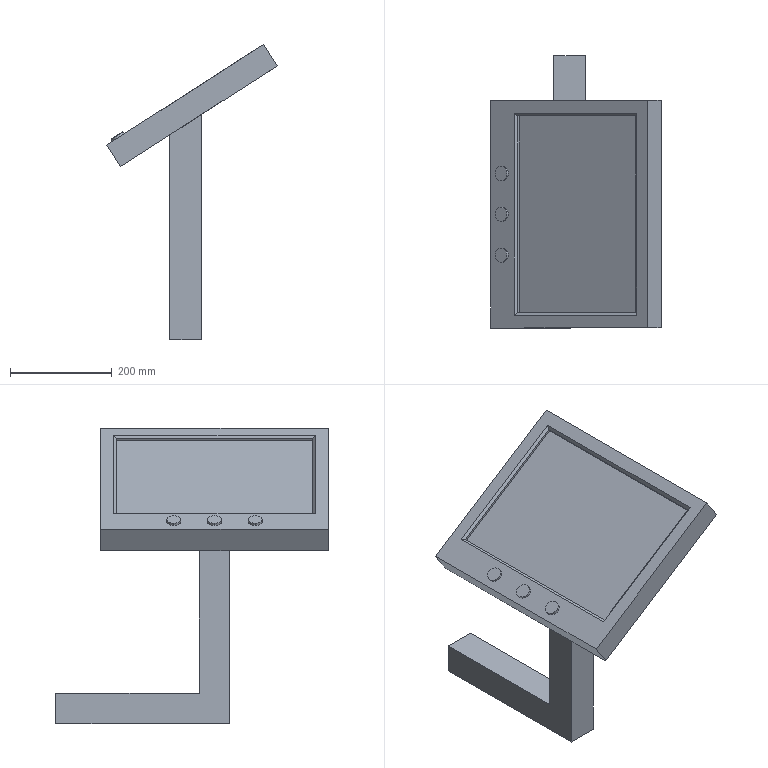Part | SolidWorks | features ICE 2, BossThin 1, Chamfer 1, Extrusion 1, MoveFace 1, Split 1 | 4 solids | 34 faces | box 334.254 x 534.204 x 579.086 mm | volume 9689433 mm3 | plane 28 | cylinder 6 | commonest cylinder face diameters 27.492 x6
STEP:
#1=CARTESIAN_POINT('',(550.446,-1023.226,1962.443));
#2=VERTEX_POINT('',#1);
#3=CARTESIAN_POINT('',(550.446,-637.226,1962.443));
#4=VERTEX_POINT('',#3);
#5=CARTESIAN_POINT('',(550.446,-637.226,1962.443));
#6=DIRECTION('',(0.,1.,0.));
#7=VECTOR('',#6,1000.);
#8=LINE('',#5,#7);
#9=EDGE_CURVE('',#2,#4,#8,.T.);
#10=ORIENTED_EDGE('',*,*,#9,.T.);
#11=CARTESIAN_POINT('',(318.933,-637.226,1813.473));
#12=VERTEX_POINT('',#11);
#13=CARTESIAN_POINT('',(550.446,-637.226,1962.443));
#14=DIRECTION('',(-0.8409,0.,-0.5411));
#15=VECTOR('',#14,1000.);
#16=LINE('',#13,#15);
#17=EDGE_CURVE('',#4,#12,#16,.T.);
#18=ORIENTED_EDGE('',*,*,#17,.T.);
#19=CARTESIAN_POINT('',(318.933,-1023.226,1813.473));
#20=VERTEX_POINT('',#19);
#21=CARTESIAN_POINT('',(318.933,-637.226,1813.473));
#22=DIRECTION('',(0.,-1.,0.));
#23=VECTOR('',#22,1000.);
#24=LINE('',#21,#23);
#25=EDGE_CURVE('',#12,#20,#24,.T.);
#26=ORIENTED_EDGE('',*,*,#25,.T.);
#27=CARTESIAN_POINT('',(550.446,-1023.226,1962.443));
#28=DIRECTION('',(0.8409,0.,0.5411));
#29=VECTOR('',#28,1000.);
#30=LINE('',#27,#29);
#31=EDGE_CURVE('',#20,#2,#30,.T.);
#32=ORIENTED_EDGE('',*,*,#31,.T.);
#33=EDGE_LOOP('',(#10,#18,#26,#32));
#34=FACE_OUTER_BOUND('',#33,.T.);
#35=CARTESIAN_POINT('',(-731.837,0.,1137.341));
#36=DIRECTION('',(0.5411,0.,-0.8409));
#37=DIRECTION('',(-0.8409,0.,-0.5411));
#38=AXIS2_PLACEMENT_3D('',#35,#36,#37);
#39=PLANE('',#38);
#40=ADVANCED_FACE('',(#34),#39,.F.);
#41=CARTESIAN_POINT('',(547.741,-1023.226,1966.648));
#42=VERTEX_POINT('',#41);
#43=CARTESIAN_POINT('',(550.446,-1023.226,1962.443));
#44=DIRECTION('',(-0.5411,0.,0.8409));
#45=VECTOR('',#44,1000.);
#46=LINE('',#43,#45);
#47=EDGE_CURVE('',#2,#42,#46,.T.);
#48=ORIENTED_EDGE('',*,*,#47,.T.);
#49=CARTESIAN_POINT('',(547.741,-637.226,1966.648));
#50=VERTEX_POINT('',#49);
#51=CARTESIAN_POINT('',(547.741,-637.226,1966.648));
#52=DIRECTION('',(0.,1.,0.));
#53=VECTOR('',#52,1000.);
#54=LINE('',#51,#53);
#55=EDGE_CURVE('',#42,#50,#54,.T.);
#56=ORIENTED_EDGE('',*,*,#55,.T.);
#57=CARTESIAN_POINT('',(550.446,-637.226,1962.443));
#58=DIRECTION('',(-0.5411,0.,0.8409));
#59=VECTOR('',#58,1000.);
#60=LINE('',#57,#59);
#61=EDGE_CURVE('',#4,#50,#60,.T.);
#62=ORIENTED_EDGE('',*,*,#61,.F.);
#63=ORIENTED_EDGE('',*,*,#9,.F.);
#64=EDGE_LOOP('',(#48,#56,#62,#63));
#65=FACE_OUTER_BOUND('',#64,.T.);
#66=CARTESIAN_POINT('',(550.446,-637.226,1962.443));
#67=DIRECTION('',(0.8409,0.,0.5411));
#68=DIRECTION('',(0.5411,0.,-0.8409));
#69=AXIS2_PLACEMENT_3D('',#66,#67,#68);
#70=PLANE('',#69);
#71=ADVANCED_FACE('',(#65),#70,.F.);
#72=ORIENTED_EDGE('',*,*,#61,.T.);
#73=CARTESIAN_POINT('',(316.227,-637.226,1817.678));
#74=VERTEX_POINT('',#73);
#75=CARTESIAN_POINT('',(316.227,-637.226,1817.678));
#76=DIRECTION('',(-0.8409,0.,-0.5411));
#77=VECTOR('',#76,1000.);
#78=LINE('',#75,#77);
#79=EDGE_CURVE('',#50,#74,#78,.T.);
#80=ORIENTED_EDGE('',*,*,#79,.T.);
#81=CARTESIAN_POINT('',(318.933,-637.226,1813.473));
#82=DIRECTION('',(-0.5411,0.,0.8409));
#83=VECTOR('',#82,1000.);
#84=LINE('',#81,#83);
#85=EDGE_CURVE('',#12,#74,#84,.T.);
#86=ORIENTED_EDGE('',*,*,#85,.F.);
#87=ORIENTED_EDGE('',*,*,#17,.F.);
#88=EDGE_LOOP('',(#72,#80,#86,#87));
#89=FACE_OUTER_BOUND('',#88,.T.);
#90=CARTESIAN_POINT('',(550.446,-637.226,1962.443));
#91=DIRECTION('',(0.,1.,0.));
#92=DIRECTION('',(0.,0.,1.));
#93=AXIS2_PLACEMENT_3D('',#90,#91,#92);
#94=PLANE('',#93);
#95=ADVANCED_FACE('',(#89),#94,.F.);
#96=CARTESIAN_POINT('',(316.227,-1023.226,1817.678));
#97=VERTEX_POINT('',#96);
#98=CARTESIAN_POINT('',(318.933,-1023.226,1813.473));
#99=DIRECTION('',(-0.5411,0.,0.8409));
#100=VECTOR('',#99,1000.);
#101=LINE('',#98,#100);
#102=EDGE_CURVE('',#20,#97,#101,.T.);
#103=ORIENTED_EDGE('',*,*,#102,.T.);
#104=CARTESIAN_POINT('',(547.741,-1023.226,1966.648));
#105=DIRECTION('',(0.8409,0.,0.5411));
#106=VECTOR('',#105,1000.);
#107=LINE('',#104,#106);
#108=EDGE_CURVE('',#97,#42,#107,.T.);
#109=ORIENTED_EDGE('',*,*,#108,.T.);
#110=ORIENTED_EDGE('',*,*,#47,.F.);
#111=ORIENTED_EDGE('',*,*,#31,.F.);
#112=EDGE_LOOP('',(#103,#109,#110,#111));
#113=FACE_OUTER_BOUND('',#112,.T.);
#114=CARTESIAN_POINT('',(550.446,-1023.226,1962.443));
#115=DIRECTION('',(0.,-1.,0.));
#116=DIRECTION('',(0.,0.,-1.));
#117=AXIS2_PLACEMENT_3D('',#114,#115,#116);
#118=PLANE('',#117);
#119=ADVANCED_FACE('',(#113),#118,.F.);
#120=CARTESIAN_POINT('',(549.24,-1028.226,1973.558));
#121=VERTEX_POINT('',#120);
#122=CARTESIAN_POINT('',(547.741,-1023.226,1966.648));
#123=DIRECTION('',(-0.1731,0.5774,-0.7979));
#124=VECTOR('',#123,1000.);
#125=LINE('',#122,#124);
#126=EDGE_CURVE('',#121,#42,#125,.T.);
#127=ORIENTED_EDGE('',*,*,#126,.F.);
#128=CARTESIAN_POINT('',(549.24,-632.226,1973.558));
#129=VERTEX_POINT('',#128);
#130=CARTESIAN_POINT('',(549.24,-1023.226,1973.558));
#131=DIRECTION('',(0.,-1.,0.));
#132=VECTOR('',#131,1000.);
#133=LINE('',#130,#132);
#134=EDGE_CURVE('',#129,#121,#133,.T.);
#135=ORIENTED_EDGE('',*,*,#134,.F.);
#136=CARTESIAN_POINT('',(547.741,-637.226,1966.648));
#137=DIRECTION('',(0.1731,0.5774,0.7979));
#138=VECTOR('',#137,1000.);
#139=LINE('',#136,#138);
#140=EDGE_CURVE('',#50,#129,#139,.T.);
#141=ORIENTED_EDGE('',*,*,#140,.F.);
#142=ORIENTED_EDGE('',*,*,#55,.F.);
#143=EDGE_LOOP('',(#127,#135,#141,#142));
#144=FACE_OUTER_BOUND('',#143,.T.);
#145=CARTESIAN_POINT('',(547.741,-637.226,1966.648));
#146=DIRECTION('',(-0.9773,0.,0.212));
#147=DIRECTION('',(0.,-1.,0.));
#148=AXIS2_PLACEMENT_3D('',#145,#146,#147);
#149=PLANE('',#148);
#150=ADVANCED_FACE('',(#144),#149,.T.);
#151=ORIENTED_EDGE('',*,*,#85,.T.);
#152=CARTESIAN_POINT('',(316.227,-1023.226,1817.678));
#153=DIRECTION('',(0.,-1.,0.));
#154=VECTOR('',#153,1000.);
#155=LINE('',#152,#154);
#156=EDGE_CURVE('',#74,#97,#155,.T.);
#157=ORIENTED_EDGE('',*,*,#156,.T.);
#158=ORIENTED_EDGE('',*,*,#102,.F.);
#159=ORIENTED_EDGE('',*,*,#25,.F.);
#160=EDGE_LOOP('',(#151,#157,#158,#159));
#161=FACE_OUTER_BOUND('',#160,.T.);
#162=CARTESIAN_POINT('',(318.933,-637.226,1813.473));
#163=DIRECTION('',(-0.8409,0.,-0.5411));
#164=DIRECTION('',(-0.5411,0.,0.8409));
#165=AXIS2_PLACEMENT_3D('',#162,#163,#164);
#166=PLANE('',#165);
#167=ADVANCED_FACE('',(#161),#166,.F.);
#168=ORIENTED_EDGE('',*,*,#126,.T.);
#169=ORIENTED_EDGE('',*,*,#108,.F.);
#170=CARTESIAN_POINT('',(309.317,-1028.226,1819.177));
#171=VERTEX_POINT('',#170);
#172=CARTESIAN_POINT('',(494.053,-894.56,1779.1));
#173=DIRECTION('',(0.7979,0.5774,-0.1731));
#174=VECTOR('',#173,1000.);
#175=LINE('',#172,#174);
#176=EDGE_CURVE('',#171,#97,#175,.T.);
#177=ORIENTED_EDGE('',*,*,#176,.F.);
#178=CARTESIAN_POINT('',(313.522,-1028.226,1821.883));
#179=DIRECTION('',(-0.8409,0.,-0.5411));
#180=VECTOR('',#179,1000.);
#181=LINE('',#178,#180);
#182=EDGE_CURVE('',#121,#171,#181,.T.);
#183=ORIENTED_EDGE('',*,*,#182,.F.);
#184=EDGE_LOOP('',(#168,#169,#177,#183));
#185=FACE_OUTER_BOUND('',#184,.T.);
#186=CARTESIAN_POINT('',(547.741,-1023.226,1966.648));
#187=DIRECTION('',(-0.3826,0.7071,0.5946));
#188=DIRECTION('',(-0.8409,0.,-0.5411));
#189=AXIS2_PLACEMENT_3D('',#186,#187,#188);
#190=PLANE('',#189);
#191=ADVANCED_FACE('',(#185),#190,.T.);
#192=ORIENTED_EDGE('',*,*,#140,.T.);
#193=CARTESIAN_POINT('',(309.317,-632.226,1819.177));
#194=VERTEX_POINT('',#193);
#195=CARTESIAN_POINT('',(545.035,-632.226,1970.853));
#196=DIRECTION('',(0.8409,0.,0.5411));
#197=VECTOR('',#196,1000.);
#198=LINE('',#195,#197);
#199=EDGE_CURVE('',#194,#129,#198,.T.);
#200=ORIENTED_EDGE('',*,*,#199,.F.);
#201=CARTESIAN_POINT('',(316.227,-637.226,1817.678));
#202=DIRECTION('',(-0.7979,0.5774,0.1731));
#203=VECTOR('',#202,1000.);
#204=LINE('',#201,#203);
#205=EDGE_CURVE('',#74,#194,#204,.T.);
#206=ORIENTED_EDGE('',*,*,#205,.F.);
#207=ORIENTED_EDGE('',*,*,#79,.F.);
#208=EDGE_LOOP('',(#192,#200,#206,#207));
#209=FACE_OUTER_BOUND('',#208,.T.);
#210=CARTESIAN_POINT('',(547.741,-637.226,1966.648));
#211=DIRECTION('',(-0.3826,-0.7071,0.5946));
#212=DIRECTION('',(0.8409,0.,0.5411));
#213=AXIS2_PLACEMENT_3D('',#210,#211,#212);
#214=PLANE('',#213);
#215=ADVANCED_FACE('',(#209),#214,.T.);
#216=ORIENTED_EDGE('',*,*,#205,.T.);
#217=CARTESIAN_POINT('',(309.317,-637.226,1819.177));
#218=DIRECTION('',(0.,1.,0.));
#219=VECTOR('',#218,1000.);
#220=LINE('',#217,#219);
#221=EDGE_CURVE('',#171,#194,#220,.T.);
#222=ORIENTED_EDGE('',*,*,#221,.F.);
#223=ORIENTED_EDGE('',*,*,#176,.T.);
#224=ORIENTED_EDGE('',*,*,#156,.F.);
#225=EDGE_LOOP('',(#216,#222,#223,#224));
#226=FACE_OUTER_BOUND('',#225,.T.);
#227=CARTESIAN_POINT('',(316.227,-637.226,1817.678));
#228=DIRECTION('',(0.212,0.,0.9773));
#229=DIRECTION('',(0.,1.,0.));
#230=AXIS2_PLACEMENT_3D('',#227,#228,#229);
#231=PLANE('',#230);
#232=ADVANCED_FACE('',(#226),#231,.T.);
#233=CARTESIAN_POINT('',(448.605,-860.226,1408.));
#234=VERTEX_POINT('',#233);
#235=CARTESIAN_POINT('',(448.605,-860.226,1849.347));
#236=VERTEX_POINT('',#235);
#237=CARTESIAN_POINT('',(448.605,-860.226,1836.321));
#238=DIRECTION('',(0.,0.,1.));
#239=VECTOR('',#238,1000.);
#240=LINE('',#237,#239);
#241=EDGE_CURVE('',#234,#236,#240,.T.);
#242=ORIENTED_EDGE('',*,*,#241,.T.);
#243=CARTESIAN_POINT('',(386.605,-860.226,1809.452));
#244=VERTEX_POINT('',#243);
#245=CARTESIAN_POINT('',(398.831,-860.226,1817.319));
#246=DIRECTION('',(0.8409,0.,0.5411));
#247=VECTOR('',#246,1000.);
#248=LINE('',#245,#247);
#249=EDGE_CURVE('',#244,#236,#248,.T.);
#250=ORIENTED_EDGE('',*,*,#249,.F.);
#251=CARTESIAN_POINT('',(386.605,-860.226,1408.));
#252=VERTEX_POINT('',#251);
#253=CARTESIAN_POINT('',(386.605,-860.226,1836.321));
#254=DIRECTION('',(0.,0.,1.));
#255=VECTOR('',#254,1000.);
#256=LINE('',#253,#255);
#257=EDGE_CURVE('',#252,#244,#256,.T.);
#258=ORIENTED_EDGE('',*,*,#257,.F.);
#259=CARTESIAN_POINT('',(386.605,-860.226,1408.));
#260=DIRECTION('',(1.,0.,0.));
#261=VECTOR('',#260,1000.);
#262=LINE('',#259,#261);
#263=EDGE_CURVE('',#252,#234,#262,.T.);
#264=ORIENTED_EDGE('',*,*,#263,.T.);
#265=EDGE_LOOP('',(#242,#250,#258,#264));
#266=FACE_OUTER_BOUND('',#265,.T.);
#267=CARTESIAN_POINT('',(386.605,-860.226,1836.321));
#268=DIRECTION('',(0.,1.,0.));
#269=DIRECTION('',(-1.,0.,0.));
#270=AXIS2_PLACEMENT_3D('',#267,#268,#269);
#271=PLANE('',#270);
#272=ADVANCED_FACE('',(#266),#271,.F.);
#273=CARTESIAN_POINT('',(448.605,-800.226,1849.347));
#274=VERTEX_POINT('',#273);
#275=CARTESIAN_POINT('',(386.605,-800.226,1809.452));
#276=VERTEX_POINT('',#275);
#277=CARTESIAN_POINT('',(231.226,-800.226,1709.472));
#278=DIRECTION('',(-0.8409,0.,-0.5411));
#279=VECTOR('',#278,1000.);
#280=LINE('',#277,#279);
#281=EDGE_CURVE('',#274,#276,#280,.T.);
#282=ORIENTED_EDGE('',*,*,#281,.F.);
#283=CARTESIAN_POINT('',(448.605,-800.226,1468.));
#284=VERTEX_POINT('',#283);
#285=CARTESIAN_POINT('',(448.605,-800.226,1468.));
#286=DIRECTION('',(0.,0.,-1.));
#287=VECTOR('',#286,1000.);
#288=LINE('',#285,#287);
#289=EDGE_CURVE('',#274,#284,#288,.T.);
#290=ORIENTED_EDGE('',*,*,#289,.T.);
#291=CARTESIAN_POINT('',(386.605,-800.226,1468.));
#292=VERTEX_POINT('',#291);
#293=CARTESIAN_POINT('',(386.605,-800.226,1468.));
#294=DIRECTION('',(1.,0.,0.));
#295=VECTOR('',#294,1000.);
#296=LINE('',#293,#295);
#297=EDGE_CURVE('',#292,#284,#296,.T.);
#298=ORIENTED_EDGE('',*,*,#297,.F.);
#299=CARTESIAN_POINT('',(386.605,-800.226,1468.));
#300=DIRECTION('',(0.,0.,-1.));
#301=VECTOR('',#300,1000.);
#302=LINE('',#299,#301);
#303=EDGE_CURVE('',#276,#292,#302,.T.);
#304=ORIENTED_EDGE('',*,*,#303,.F.);
#305=EDGE_LOOP('',(#282,#290,#298,#304));
#306=FACE_OUTER_BOUND('',#305,.T.);
#307=CARTESIAN_POINT('',(386.605,-800.226,1468.));
#308=DIRECTION('',(0.,-1.,0.));
#309=DIRECTION('',(1.,0.,0.));
#310=AXIS2_PLACEMENT_3D('',#307,#308,#309);
#311=PLANE('',#310);
#312=ADVANCED_FACE('',(#306),#311,.F.);
#313=CARTESIAN_POINT('',(386.605,0.,1809.452));
#314=DIRECTION('',(0.,-1.,0.));
#315=VECTOR('',#314,1000.);
#316=LINE('',#313,#315);
#317=EDGE_CURVE('',#276,#244,#316,.T.);
#318=ORIENTED_EDGE('',*,*,#317,.F.);
#319=ORIENTED_EDGE('',*,*,#303,.T.);
#320=CARTESIAN_POINT('',(386.605,-519.023,1468.));
#321=VERTEX_POINT('',#320);
#322=CARTESIAN_POINT('',(386.605,-519.023,1468.));
#323=DIRECTION('',(0.,1.,0.));
#324=VECTOR('',#323,1000.);
#325=LINE('',#322,#324);
#326=EDGE_CURVE('',#292,#321,#325,.T.);
#327=ORIENTED_EDGE('',*,*,#326,.T.);
#328=CARTESIAN_POINT('',(386.605,-519.023,1408.));
#329=VERTEX_POINT('',#328);
#330=CARTESIAN_POINT('',(386.605,-519.023,1468.));
#331=DIRECTION('',(0.,0.,-1.));
#332=VECTOR('',#331,1000.);
#333=LINE('',#330,#332);
#334=EDGE_CURVE('',#321,#329,#333,.T.);
#335=ORIENTED_EDGE('',*,*,#334,.T.);
#336=CARTESIAN_POINT('',(386.605,-860.226,1408.));
#337=DIRECTION('',(0.,-1.,0.));
#338=VECTOR('',#337,1000.);
#339=LINE('',#336,#338);
#340=EDGE_CURVE('',#329,#252,#339,.T.);
#341=ORIENTED_EDGE('',*,*,#340,.T.);
#342=ORIENTED_EDGE('',*,*,#257,.T.);
#343=EDGE_LOOP('',(#318,#319,#327,#335,#341,#342));
#344=FACE_OUTER_BOUND('',#343,.T.);
#345=CARTESIAN_POINT('',(386.605,0.,0.));
#346=DIRECTION('',(1.,0.,0.));
#347=DIRECTION('',(0.,0.,-1.));
#348=AXIS2_PLACEMENT_3D('',#345,#346,#347);
#349=PLANE('',#348);
#350=ADVANCED_FACE('',(#344),#349,.F.);
#351=CARTESIAN_POINT('',(448.605,-519.023,1468.));
#352=VERTEX_POINT('',#351);
#353=CARTESIAN_POINT('',(448.605,-519.023,1408.));
#354=VERTEX_POINT('',#353);
#355=CARTESIAN_POINT('',(448.605,-519.023,1468.));
#356=DIRECTION('',(0.,0.,-1.));
#357=VECTOR('',#356,1000.);
#358=LINE('',#355,#357);
#359=EDGE_CURVE('',#352,#354,#358,.T.);
#360=ORIENTED_EDGE('',*,*,#359,.T.);
#361=CARTESIAN_POINT('',(386.605,-519.023,1408.));
#362=DIRECTION('',(1.,0.,0.));
#363=VECTOR('',#362,1000.);
#364=LINE('',#361,#363);
#365=EDGE_CURVE('',#329,#354,#364,.T.);
#366=ORIENTED_EDGE('',*,*,#365,.F.);
#367=ORIENTED_EDGE('',*,*,#334,.F.);
#368=CARTESIAN_POINT('',(386.605,-519.023,1468.));
#369=DIRECTION('',(1.,0.,0.));
#370=VECTOR('',#369,1000.);
#371=LINE('',#368,#370);
#372=EDGE_CURVE('',#321,#352,#371,.T.);
#373=ORIENTED_EDGE('',*,*,#372,.T.);
#374=EDGE_LOOP('',(#360,#366,#367,#373));
#375=FACE_OUTER_BOUND('',#374,.T.);
#376=CARTESIAN_POINT('',(386.605,-519.023,1468.));
#377=DIRECTION('',(0.,-1.,0.));
#378=DIRECTION('',(1.,0.,0.));
#379=AXIS2_PLACEMENT_3D('',#376,#377,#378);
#380=PLANE('',#379);
#381=ADVANCED_FACE('',(#375),#380,.F.);
#382=CARTESIAN_POINT('',(448.605,-860.226,1408.));
#383=DIRECTION('',(0.,-1.,0.));
#384=VECTOR('',#383,1000.);
#385=LINE('',#382,#384);
#386=EDGE_CURVE('',#354,#234,#385,.T.);
#387=ORIENTED_EDGE('',*,*,#386,.T.);
#388=ORIENTED_EDGE('',*,*,#263,.F.);
#389=ORIENTED_EDGE('',*,*,#340,.F.);
#390=ORIENTED_EDGE('',*,*,#365,.T.);
#391=EDGE_LOOP('',(#387,#388,#389,#390));
#392=FACE_OUTER_BOUND('',#391,.T.);
#393=CARTESIAN_POINT('',(386.605,-860.226,1408.));
#394=DIRECTION('',(0.,0.,1.));
#395=DIRECTION('',(0.,-1.,0.));
#396=AXIS2_PLACEMENT_3D('',#393,#394,#395);
#397=PLANE('',#396);
#398=ADVANCED_FACE('',(#392),#397,.F.);
#399=CARTESIAN_POINT('',(448.605,-519.023,1468.));
#400=DIRECTION('',(0.,1.,0.));
#401=VECTOR('',#400,1000.);
#402=LINE('',#399,#401);
#403=EDGE_CURVE('',#284,#352,#402,.T.);
#404=ORIENTED_EDGE('',*,*,#403,.T.);
#405=ORIENTED_EDGE('',*,*,#372,.F.);
#406=ORIENTED_EDGE('',*,*,#326,.F.);
#407=ORIENTED_EDGE('',*,*,#297,.T.);
#408=EDGE_LOOP('',(#404,#405,#406,#407));
#409=FACE_OUTER_BOUND('',#408,.T.);
#410=CARTESIAN_POINT('',(386.605,-519.023,1468.));
#411=DIRECTION('',(0.,0.,-1.));
#412=DIRECTION('',(-1.,0.,0.));
#413=AXIS2_PLACEMENT_3D('',#410,#411,#412);
#414=PLANE('',#413);
#415=ADVANCED_FACE('',(#409),#414,.F.);
#416=ORIENTED_EDGE('',*,*,#359,.F.);
#417=ORIENTED_EDGE('',*,*,#403,.F.);
#418=ORIENTED_EDGE('',*,*,#289,.F.);
#419=CARTESIAN_POINT('',(448.605,-1053.226,1849.347));
#420=DIRECTION('',(0.,-1.,0.));
#421=VECTOR('',#420,1000.);
#422=LINE('',#419,#421);
#423=EDGE_CURVE('',#274,#236,#422,.T.);
#424=ORIENTED_EDGE('',*,*,#423,.T.);
#425=ORIENTED_EDGE('',*,*,#241,.F.);
#426=ORIENTED_EDGE('',*,*,#386,.F.);
#427=EDGE_LOOP('',(#416,#417,#418,#424,#425,#426));
#428=FACE_OUTER_BOUND('',#427,.T.);
#429=CARTESIAN_POINT('',(448.605,0.,0.));
#430=DIRECTION('',(1.,0.,0.));
#431=DIRECTION('',(0.,0.,-1.));
#432=AXIS2_PLACEMENT_3D('',#429,#430,#431);
#433=PLANE('',#432);
#434=ADVANCED_FACE('',(#428),#433,.T.);
#435=CARTESIAN_POINT('',(290.121,-607.226,1747.368));
#436=VERTEX_POINT('',#435);
#437=CARTESIAN_POINT('',(597.319,-607.226,1945.039));
#438=VERTEX_POINT('',#437);
#439=CARTESIAN_POINT('',(290.121,-607.226,1747.368));
#440=DIRECTION('',(0.8409,0.,0.5411));
#441=VECTOR('',#440,1000.);
#442=LINE('',#439,#441);
#443=EDGE_CURVE('',#436,#438,#442,.T.);
#444=ORIENTED_EDGE('',*,*,#443,.T.);
#445=CARTESIAN_POINT('',(597.319,-1053.226,1945.039));
#446=VERTEX_POINT('',#445);
#447=CARTESIAN_POINT('',(597.319,-1053.226,1945.039));
#448=DIRECTION('',(0.,1.,0.));
#449=VECTOR('',#448,1000.);
#450=LINE('',#447,#449);
#451=EDGE_CURVE('',#446,#438,#450,.T.);
#452=ORIENTED_EDGE('',*,*,#451,.F.);
#453=CARTESIAN_POINT('',(290.121,-1053.226,1747.368));
#454=VERTEX_POINT('',#453);
#455=CARTESIAN_POINT('',(290.121,-1053.226,1747.368));
#456=DIRECTION('',(0.8409,0.,0.5411));
#457=VECTOR('',#456,1000.);
#458=LINE('',#455,#457);
#459=EDGE_CURVE('',#454,#446,#458,.T.);
#460=ORIENTED_EDGE('',*,*,#459,.F.);
#461=CARTESIAN_POINT('',(290.121,-1053.226,1747.368));
#462=DIRECTION('',(0.,1.,0.));
#463=VECTOR('',#462,1000.);
#464=LINE('',#461,#463);
#465=EDGE_CURVE('',#454,#436,#464,.T.);
#466=ORIENTED_EDGE('',*,*,#465,.T.);
#467=EDGE_LOOP('',(#444,#452,#460,#466));
#468=FACE_OUTER_BOUND('',#467,.T.);
#469=ORIENTED_EDGE('',*,*,#317,.T.);
#470=ORIENTED_EDGE('',*,*,#249,.T.);
#471=ORIENTED_EDGE('',*,*,#423,.F.);
#472=ORIENTED_EDGE('',*,*,#281,.T.);
#473=EDGE_LOOP('',(#469,#470,#471,#472));
#474=FACE_BOUND('',#473,.T.);
#475=CARTESIAN_POINT('',(290.121,-1053.226,1747.368));
#476=DIRECTION('',(-0.5411,0.,0.8409));
#477=DIRECTION('',(0.8409,0.,0.5411));
#478=AXIS2_PLACEMENT_3D('',#475,#476,#477);
#479=PLANE('',#478);
#480=ADVANCED_FACE('',(#468,#474),#479,.F.);
#481=CARTESIAN_POINT('',(570.263,-607.226,1987.086));
#482=VERTEX_POINT('',#481);
#483=CARTESIAN_POINT('',(570.263,-607.226,1987.086));
#484=DIRECTION('',(0.5411,0.,-0.8409));
#485=VECTOR('',#484,1000.);
#486=LINE('',#483,#485);
#487=EDGE_CURVE('',#482,#438,#486,.T.);
#488=ORIENTED_EDGE('',*,*,#487,.F.);
#489=CARTESIAN_POINT('',(570.263,-1053.226,1987.086));
#490=VERTEX_POINT('',#489);
#491=CARTESIAN_POINT('',(570.263,-1053.226,1987.086));
#492=DIRECTION('',(0.,1.,0.));
#493=VECTOR('',#492,1000.);
#494=LINE('',#491,#493);
#495=EDGE_CURVE('',#490,#482,#494,.T.);
#496=ORIENTED_EDGE('',*,*,#495,.F.);
#497=CARTESIAN_POINT('',(570.263,-1053.226,1987.086));
#498=DIRECTION('',(0.5411,0.,-0.8409));
#499=VECTOR('',#498,1000.);
#500=LINE('',#497,#499);
#501=EDGE_CURVE('',#490,#446,#500,.T.);
#502=ORIENTED_EDGE('',*,*,#501,.T.);
#503=ORIENTED_EDGE('',*,*,#451,.T.);
#504=EDGE_LOOP('',(#488,#496,#502,#503));
#505=FACE_OUTER_BOUND('',#504,.T.);
#506=CARTESIAN_POINT('',(570.263,-1053.226,1987.086));
#507=DIRECTION('',(0.8409,0.,0.5411));
#508=DIRECTION('',(0.5411,0.,-0.8409));
#509=AXIS2_PLACEMENT_3D('',#506,#507,#508);
#510=PLANE('',#509);
#511=ADVANCED_FACE('',(#505),#510,.T.);
#512=CARTESIAN_POINT('',(263.065,-607.226,1789.415));
#513=VERTEX_POINT('',#512);
#514=CARTESIAN_POINT('',(290.121,-607.226,1747.368));
#515=DIRECTION('',(-0.5411,0.,0.8409));
#516=VECTOR('',#515,1000.);
#517=LINE('',#514,#516);
#518=EDGE_CURVE('',#436,#513,#517,.T.);
#519=ORIENTED_EDGE('',*,*,#518,.F.);
#520=ORIENTED_EDGE('',*,*,#465,.F.);
#521=CARTESIAN_POINT('',(263.065,-1053.226,1789.415));
#522=VERTEX_POINT('',#521);
#523=CARTESIAN_POINT('',(290.121,-1053.226,1747.368));
#524=DIRECTION('',(-0.5411,0.,0.8409));
#525=VECTOR('',#524,1000.);
#526=LINE('',#523,#525);
#527=EDGE_CURVE('',#454,#522,#526,.T.);
#528=ORIENTED_EDGE('',*,*,#527,.T.);
#529=CARTESIAN_POINT('',(263.065,-1053.226,1789.415));
#530=DIRECTION('',(0.,1.,0.));
#531=VECTOR('',#530,1000.);
#532=LINE('',#529,#531);
#533=EDGE_CURVE('',#522,#513,#532,.T.);
#534=ORIENTED_EDGE('',*,*,#533,.T.);
#535=EDGE_LOOP('',(#519,#520,#528,#534));
#536=FACE_OUTER_BOUND('',#535,.T.);
#537=CARTESIAN_POINT('',(290.121,-1053.226,1747.368));
#538=DIRECTION('',(-0.8409,0.,-0.5411));
#539=DIRECTION('',(-0.5411,0.,0.8409));
#540=AXIS2_PLACEMENT_3D('',#537,#538,#539);
#541=PLANE('',#540);
#542=ADVANCED_FACE('',(#536),#541,.T.);
#543=ORIENTED_EDGE('',*,*,#459,.T.);
#544=ORIENTED_EDGE('',*,*,#501,.F.);
#545=CARTESIAN_POINT('',(263.065,-1053.226,1789.415));
#546=DIRECTION('',(0.8409,0.,0.5411));
#547=VECTOR('',#546,1000.);
#548=LINE('',#545,#547);
#549=EDGE_CURVE('',#522,#490,#548,.T.);
#550=ORIENTED_EDGE('',*,*,#549,.F.);
#551=ORIENTED_EDGE('',*,*,#527,.F.);
#552=EDGE_LOOP('',(#543,#544,#550,#551));
#553=FACE_OUTER_BOUND('',#552,.T.);
#554=CARTESIAN_POINT('',(0.,-1053.226,0.));
#555=DIRECTION('',(0.,1.,0.));
#556=DIRECTION('',(1.,0.,0.));
#557=AXIS2_PLACEMENT_3D('',#554,#555,#556);
#558=PLANE('',#557);
#559=ADVANCED_FACE('',(#553),#558,.F.);
#560=ORIENTED_EDGE('',*,*,#443,.F.);
#561=ORIENTED_EDGE('',*,*,#518,.T.);
#562=CARTESIAN_POINT('',(263.065,-607.226,1789.415));
#563=DIRECTION('',(0.8409,0.,0.5411));
#564=VECTOR('',#563,1000.);
#565=LINE('',#562,#564);
#566=EDGE_CURVE('',#513,#482,#565,.T.);
#567=ORIENTED_EDGE('',*,*,#566,.T.);
#568=ORIENTED_EDGE('',*,*,#487,.T.);
#569=EDGE_LOOP('',(#560,#561,#567,#568));
#570=FACE_OUTER_BOUND('',#569,.T.);
#571=CARTESIAN_POINT('',(0.,-607.226,0.));
#572=DIRECTION('',(0.,1.,0.));
#573=DIRECTION('',(1.,0.,0.));
#574=AXIS2_PLACEMENT_3D('',#571,#572,#573);
#575=PLANE('',#574);
#576=ADVANCED_FACE('',(#570),#575,.T.);
#577=ORIENTED_EDGE('',*,*,#182,.T.);
#578=ORIENTED_EDGE('',*,*,#221,.T.);
#579=ORIENTED_EDGE('',*,*,#199,.T.);
#580=ORIENTED_EDGE('',*,*,#134,.T.);
#581=EDGE_LOOP('',(#577,#578,#579,#580));
#582=FACE_BOUND('',#581,.T.);
#583=ORIENTED_EDGE('',*,*,#566,.F.);
#584=ORIENTED_EDGE('',*,*,#533,.F.);
#585=ORIENTED_EDGE('',*,*,#549,.T.);
#586=ORIENTED_EDGE('',*,*,#495,.T.);
#587=EDGE_LOOP('',(#583,#584,#585,#586));
#588=FACE_OUTER_BOUND('',#587,.T.);
#589=CARTESIAN_POINT('',(263.065,-607.226,1789.415));
#590=DIRECTION('',(-0.5411,0.,0.8409));
#591=DIRECTION('',(0.8409,0.,0.5411));
#592=AXIS2_PLACEMENT_3D('',#589,#590,#591);
#593=PLANE('',#592);
#594=ADVANCED_FACE('',(#582,#588),#593,.T.);
#595=CLOSED_SHELL('',(#40,#71,#95,#119,#150,#167,#191,#215,#232,#272,#312,#350,#381,#398,#415,#434,#480,#511,#542,#559,#576,#594));
#596=MANIFOLD_SOLID_BREP('',#595);
#597=CARTESIAN_POINT('',(294.535,-750.226,1815.611));
#598=VERTEX_POINT('',#597);
#599=CARTESIAN_POINT('',(271.416,-750.226,1800.735));
#600=VERTEX_POINT('',#599);
#601=CARTESIAN_POINT('',(282.976,-750.226,1808.173));
#602=DIRECTION('',(-0.5411,0.,0.8409));
#603=DIRECTION('',(0.8409,0.,0.5411));
#604=AXIS2_PLACEMENT_3D('',#601,#602,#603);
#605=CIRCLE('',#604,13.746);
#606=EDGE_CURVE('',#598,#600,#605,.T.);
#607=ORIENTED_EDGE('',*,*,#606,.F.);
#608=CARTESIAN_POINT('',(297.241,-750.226,1811.406));
#609=VERTEX_POINT('',#608);
#610=CARTESIAN_POINT('',(294.535,-750.226,1815.611));
#611=DIRECTION('',(0.5411,0.,-0.8409));
#612=VECTOR('',#611,1000.);
#613=LINE('',#610,#612);
#614=EDGE_CURVE('',#598,#609,#613,.T.);
#615=ORIENTED_EDGE('',*,*,#614,.T.);
#616=CARTESIAN_POINT('',(274.121,-750.226,1796.53));
#617=VERTEX_POINT('',#616);
#618=CARTESIAN_POINT('',(285.681,-750.226,1803.968));
#619=DIRECTION('',(-0.5411,0.,0.8409));
#620=DIRECTION('',(0.8409,0.,0.5411));
#621=AXIS2_PLACEMENT_3D('',#618,#619,#620);
#622=CIRCLE('',#621,13.746);
#623=EDGE_CURVE('',#609,#617,#622,.T.);
#624=ORIENTED_EDGE('',*,*,#623,.T.);
#625=CARTESIAN_POINT('',(271.416,-750.226,1800.735));
#626=DIRECTION('',(0.5411,0.,-0.8409));
#627=VECTOR('',#626,1000.);
#628=LINE('',#625,#627);
#629=EDGE_CURVE('',#600,#617,#628,.T.);
#630=ORIENTED_EDGE('',*,*,#629,.F.);
#631=EDGE_LOOP('',(#607,#615,#624,#630));
#632=FACE_OUTER_BOUND('',#631,.T.);
#633=CARTESIAN_POINT('',(282.976,-750.226,1808.173));
#634=DIRECTION('',(0.5411,0.,-0.8409));
#635=DIRECTION('',(-0.8409,0.,-0.5411));
#636=AXIS2_PLACEMENT_3D('',#633,#634,#635);
#637=CYLINDRICAL_SURFACE('',#636,13.746);
#638=ADVANCED_FACE('',(#632),#637,.T.);
#639=CARTESIAN_POINT('',(285.681,-750.226,1803.968));
#640=DIRECTION('',(-0.5411,0.,0.8409));
#641=DIRECTION('',(0.8409,0.,0.5411));
#642=AXIS2_PLACEMENT_3D('',#639,#640,#641);
#643=CIRCLE('',#642,13.746);
#644=EDGE_CURVE('',#617,#609,#643,.T.);
#645=ORIENTED_EDGE('',*,*,#644,.F.);
#646=ORIENTED_EDGE('',*,*,#623,.F.);
#647=EDGE_LOOP('',(#645,#646));
#648=FACE_OUTER_BOUND('',#647,.T.);
#649=CARTESIAN_POINT('',(263.065,-607.226,1789.415));
#650=DIRECTION('',(-0.5411,0.,0.8409));
#651=DIRECTION('',(0.8409,0.,0.5411));
#652=AXIS2_PLACEMENT_3D('',#649,#650,#651);
#653=PLANE('',#652);
#654=ADVANCED_FACE('',(#648),#653,.F.);
#655=ORIENTED_EDGE('',*,*,#614,.F.);
#656=CARTESIAN_POINT('',(282.976,-750.226,1808.173));
#657=DIRECTION('',(-0.5411,0.,0.8409));
#658=DIRECTION('',(0.8409,0.,0.5411));
#659=AXIS2_PLACEMENT_3D('',#656,#657,#658);
#660=CIRCLE('',#659,13.746);
#661=EDGE_CURVE('',#600,#598,#660,.T.);
#662=ORIENTED_EDGE('',*,*,#661,.F.);
#663=ORIENTED_EDGE('',*,*,#629,.T.);
#664=ORIENTED_EDGE('',*,*,#644,.T.);
#665=EDGE_LOOP('',(#655,#662,#663,#664));
#666=FACE_OUTER_BOUND('',#665,.T.);
#667=CARTESIAN_POINT('',(282.976,-750.226,1808.173));
#668=DIRECTION('',(0.5411,0.,-0.8409));
#669=DIRECTION('',(-0.8409,0.,-0.5411));
#670=AXIS2_PLACEMENT_3D('',#667,#668,#669);
#671=CYLINDRICAL_SURFACE('',#670,13.746);
#672=ADVANCED_FACE('',(#666),#671,.T.);
#673=ORIENTED_EDGE('',*,*,#661,.T.);
#674=ORIENTED_EDGE('',*,*,#606,.T.);
#675=EDGE_LOOP('',(#673,#674));
#676=FACE_OUTER_BOUND('',#675,.T.);
#677=CARTESIAN_POINT('',(282.976,-750.226,1808.173));
#678=DIRECTION('',(-0.5411,0.,0.8409));
#679=DIRECTION('',(0.8409,0.,0.5411));
#680=AXIS2_PLACEMENT_3D('',#677,#678,#679);
#681=PLANE('',#680);
#682=ADVANCED_FACE('',(#676),#681,.T.);
#683=CLOSED_SHELL('',(#638,#654,#672,#682));
#684=MANIFOLD_SOLID_BREP('',#683);
#685=CARTESIAN_POINT('',(294.535,-830.226,1815.611));
#686=VERTEX_POINT('',#685);
#687=CARTESIAN_POINT('',(271.416,-830.226,1800.735));
#688=VERTEX_POINT('',#687);
#689=CARTESIAN_POINT('',(282.976,-830.226,1808.173));
#690=DIRECTION('',(-0.5411,0.,0.8409));
#691=DIRECTION('',(0.8409,0.,0.5411));
#692=AXIS2_PLACEMENT_3D('',#689,#690,#691);
#693=CIRCLE('',#692,13.746);
#694=EDGE_CURVE('',#686,#688,#693,.T.);
#695=ORIENTED_EDGE('',*,*,#694,.F.);
#696=CARTESIAN_POINT('',(297.241,-830.226,1811.406));
#697=VERTEX_POINT('',#696);
#698=CARTESIAN_POINT('',(294.535,-830.226,1815.611));
#699=DIRECTION('',(0.5411,0.,-0.8409));
#700=VECTOR('',#699,1000.);
#701=LINE('',#698,#700);
#702=EDGE_CURVE('',#686,#697,#701,.T.);
#703=ORIENTED_EDGE('',*,*,#702,.T.);
#704=CARTESIAN_POINT('',(274.121,-830.226,1796.53));
#705=VERTEX_POINT('',#704);
#706=CARTESIAN_POINT('',(285.681,-830.226,1803.968));
#707=DIRECTION('',(-0.5411,0.,0.8409));
#708=DIRECTION('',(0.8409,0.,0.5411));
#709=AXIS2_PLACEMENT_3D('',#706,#707,#708);
#710=CIRCLE('',#709,13.746);
#711=EDGE_CURVE('',#697,#705,#710,.T.);
#712=ORIENTED_EDGE('',*,*,#711,.T.);
#713=CARTESIAN_POINT('',(271.416,-830.226,1800.735));
#714=DIRECTION('',(0.5411,0.,-0.8409));
#715=VECTOR('',#714,1000.);
#716=LINE('',#713,#715);
#717=EDGE_CURVE('',#688,#705,#716,.T.);
#718=ORIENTED_EDGE('',*,*,#717,.F.);
#719=EDGE_LOOP('',(#695,#703,#712,#718));
#720=FACE_OUTER_BOUND('',#719,.T.);
#721=CARTESIAN_POINT('',(282.976,-830.226,1808.173));
#722=DIRECTION('',(0.5411,0.,-0.8409));
#723=DIRECTION('',(-0.8409,0.,-0.5411));
#724=AXIS2_PLACEMENT_3D('',#721,#722,#723);
#725=CYLINDRICAL_SURFACE('',#724,13.746);
#726=ADVANCED_FACE('',(#720),#725,.T.);
#727=CARTESIAN_POINT('',(285.681,-830.226,1803.968));
#728=DIRECTION('',(-0.5411,0.,0.8409));
#729=DIRECTION('',(0.8409,0.,0.5411));
#730=AXIS2_PLACEMENT_3D('',#727,#728,#729);
#731=CIRCLE('',#730,13.746);
#732=EDGE_CURVE('',#705,#697,#731,.T.);
#733=ORIENTED_EDGE('',*,*,#732,.F.);
#734=ORIENTED_EDGE('',*,*,#711,.F.);
#735=EDGE_LOOP('',(#733,#734));
#736=FACE_OUTER_BOUND('',#735,.T.);
#737=CARTESIAN_POINT('',(263.065,-607.226,1789.415));
#738=DIRECTION('',(-0.5411,0.,0.8409));
#739=DIRECTION('',(0.8409,0.,0.5411));
#740=AXIS2_PLACEMENT_3D('',#737,#738,#739);
#741=PLANE('',#740);
#742=ADVANCED_FACE('',(#736),#741,.F.);
#743=ORIENTED_EDGE('',*,*,#702,.F.);
#744=CARTESIAN_POINT('',(282.976,-830.226,1808.173));
#745=DIRECTION('',(-0.5411,0.,0.8409));
#746=DIRECTION('',(0.8409,0.,0.5411));
#747=AXIS2_PLACEMENT_3D('',#744,#745,#746);
#748=CIRCLE('',#747,13.746);
#749=EDGE_CURVE('',#688,#686,#748,.T.);
#750=ORIENTED_EDGE('',*,*,#749,.F.);
#751=ORIENTED_EDGE('',*,*,#717,.T.);
#752=ORIENTED_EDGE('',*,*,#732,.T.);
#753=EDGE_LOOP('',(#743,#750,#751,#752));
#754=FACE_OUTER_BOUND('',#753,.T.);
#755=CARTESIAN_POINT('',(282.976,-830.226,1808.173));
#756=DIRECTION('',(0.5411,0.,-0.8409));
#757=DIRECTION('',(-0.8409,0.,-0.5411));
#758=AXIS2_PLACEMENT_3D('',#755,#756,#757);
#759=CYLINDRICAL_SURFACE('',#758,13.746);
#760=ADVANCED_FACE('',(#754),#759,.T.);
#761=ORIENTED_EDGE('',*,*,#749,.T.);
#762=ORIENTED_EDGE('',*,*,#694,.T.);
#763=EDGE_LOOP('',(#761,#762));
#764=FACE_OUTER_BOUND('',#763,.T.);
#765=CARTESIAN_POINT('',(282.976,-830.226,1808.173));
#766=DIRECTION('',(-0.5411,0.,0.8409));
#767=DIRECTION('',(0.8409,0.,0.5411));
#768=AXIS2_PLACEMENT_3D('',#765,#766,#767);
#769=PLANE('',#768);
#770=ADVANCED_FACE('',(#764),#769,.T.);
#771=CLOSED_SHELL('',(#726,#742,#760,#770));
#772=MANIFOLD_SOLID_BREP('',#771);
#773=CARTESIAN_POINT('',(294.535,-910.226,1815.611));
#774=VERTEX_POINT('',#773);
#775=CARTESIAN_POINT('',(271.416,-910.226,1800.735));
#776=VERTEX_POINT('',#775);
#777=CARTESIAN_POINT('',(282.976,-910.226,1808.173));
#778=DIRECTION('',(-0.5411,0.,0.8409));
#779=DIRECTION('',(0.8409,0.,0.5411));
#780=AXIS2_PLACEMENT_3D('',#777,#778,#779);
#781=CIRCLE('',#780,13.746);
#782=EDGE_CURVE('',#774,#776,#781,.T.);
#783=ORIENTED_EDGE('',*,*,#782,.F.);
#784=CARTESIAN_POINT('',(297.241,-910.226,1811.406));
#785=VERTEX_POINT('',#784);
#786=CARTESIAN_POINT('',(294.535,-910.226,1815.611));
#787=DIRECTION('',(0.5411,0.,-0.8409));
#788=VECTOR('',#787,1000.);
#789=LINE('',#786,#788);
#790=EDGE_CURVE('',#774,#785,#789,.T.);
#791=ORIENTED_EDGE('',*,*,#790,.T.);
#792=CARTESIAN_POINT('',(274.121,-910.226,1796.53));
#793=VERTEX_POINT('',#792);
#794=CARTESIAN_POINT('',(285.681,-910.226,1803.968));
#795=DIRECTION('',(-0.5411,0.,0.8409));
#796=DIRECTION('',(0.8409,0.,0.5411));
#797=AXIS2_PLACEMENT_3D('',#794,#795,#796);
#798=CIRCLE('',#797,13.746);
#799=EDGE_CURVE('',#785,#793,#798,.T.);
#800=ORIENTED_EDGE('',*,*,#799,.T.);
#801=CARTESIAN_POINT('',(271.416,-910.226,1800.735));
#802=DIRECTION('',(0.5411,0.,-0.8409));
#803=VECTOR('',#802,1000.);
#804=LINE('',#801,#803);
#805=EDGE_CURVE('',#776,#793,#804,.T.);
#806=ORIENTED_EDGE('',*,*,#805,.F.);
#807=EDGE_LOOP('',(#783,#791,#800,#806));
#808=FACE_OUTER_BOUND('',#807,.T.);
#809=CARTESIAN_POINT('',(282.976,-910.226,1808.173));
#810=DIRECTION('',(0.5411,0.,-0.8409));
#811=DIRECTION('',(-0.8409,0.,-0.5411));
#812=AXIS2_PLACEMENT_3D('',#809,#810,#811);
#813=CYLINDRICAL_SURFACE('',#812,13.746);
#814=ADVANCED_FACE('',(#808),#813,.T.);
#815=CARTESIAN_POINT('',(285.681,-910.226,1803.968));
#816=DIRECTION('',(-0.5411,0.,0.8409));
#817=DIRECTION('',(0.8409,0.,0.5411));
#818=AXIS2_PLACEMENT_3D('',#815,#816,#817);
#819=CIRCLE('',#818,13.746);
#820=EDGE_CURVE('',#793,#785,#819,.T.);
#821=ORIENTED_EDGE('',*,*,#820,.F.);
#822=ORIENTED_EDGE('',*,*,#799,.F.);
#823=EDGE_LOOP('',(#821,#822));
#824=FACE_OUTER_BOUND('',#823,.T.);
#825=CARTESIAN_POINT('',(263.065,-607.226,1789.415));
#826=DIRECTION('',(-0.5411,0.,0.8409));
#827=DIRECTION('',(0.8409,0.,0.5411));
#828=AXIS2_PLACEMENT_3D('',#825,#826,#827);
#829=PLANE('',#828);
#830=ADVANCED_FACE('',(#824),#829,.F.);
#831=ORIENTED_EDGE('',*,*,#790,.F.);
#832=CARTESIAN_POINT('',(282.976,-910.226,1808.173));
#833=DIRECTION('',(-0.5411,0.,0.8409));
#834=DIRECTION('',(0.8409,0.,0.5411));
#835=AXIS2_PLACEMENT_3D('',#832,#833,#834);
#836=CIRCLE('',#835,13.746);
#837=EDGE_CURVE('',#776,#774,#836,.T.);
#838=ORIENTED_EDGE('',*,*,#837,.F.);
#839=ORIENTED_EDGE('',*,*,#805,.T.);
#840=ORIENTED_EDGE('',*,*,#820,.T.);
#841=EDGE_LOOP('',(#831,#838,#839,#840));
#842=FACE_OUTER_BOUND('',#841,.T.);
#843=CARTESIAN_POINT('',(282.976,-910.226,1808.173));
#844=DIRECTION('',(0.5411,0.,-0.8409));
#845=DIRECTION('',(-0.8409,0.,-0.5411));
#846=AXIS2_PLACEMENT_3D('',#843,#844,#845);
#847=CYLINDRICAL_SURFACE('',#846,13.746);
#848=ADVANCED_FACE('',(#842),#847,.T.);
#849=ORIENTED_EDGE('',*,*,#837,.T.);
#850=ORIENTED_EDGE('',*,*,#782,.T.);
#851=EDGE_LOOP('',(#849,#850));
#852=FACE_OUTER_BOUND('',#851,.T.);
#853=CARTESIAN_POINT('',(282.976,-910.226,1808.173));
#854=DIRECTION('',(-0.5411,0.,0.8409));
#855=DIRECTION('',(0.8409,0.,0.5411));
#856=AXIS2_PLACEMENT_3D('',#853,#854,#855);
#857=PLANE('',#856);
#858=ADVANCED_FACE('',(#852),#857,.T.);
#859=CLOSED_SHELL('',(#814,#830,#848,#858));
#860=MANIFOLD_SOLID_BREP('',#859);
#861=CARTESIAN_POINT('',(0.,0.,0.));
#862=DIRECTION('',(0.,0.,1.));
#863=DIRECTION('',(1.,0.,0.));
#864=AXIS2_PLACEMENT_3D('',#861,#862,#863);
#865=(LENGTH_UNIT()NAMED_UNIT(*)SI_UNIT(.MILLI.,.METRE.));
#866=UNCERTAINTY_MEASURE_WITH_UNIT(LENGTH_MEASURE(0.00001),#865,'','');
#867=(NAMED_UNIT(*)PLANE_ANGLE_UNIT()SI_UNIT($,.RADIAN.));
#868=(NAMED_UNIT(*)SI_UNIT($,.STERADIAN.)SOLID_ANGLE_UNIT());
#869=(GEOMETRIC_REPRESENTATION_CONTEXT(3)GLOBAL_UNCERTAINTY_ASSIGNED_CONTEXT((#866))GLOBAL_UNIT_ASSIGNED_CONTEXT((#865,#867,#868))REPRESENTATION_CONTEXT('',''));
#870=ADVANCED_BREP_SHAPE_REPRESENTATION('',(#596,#684,#772,#860,#864),#869);